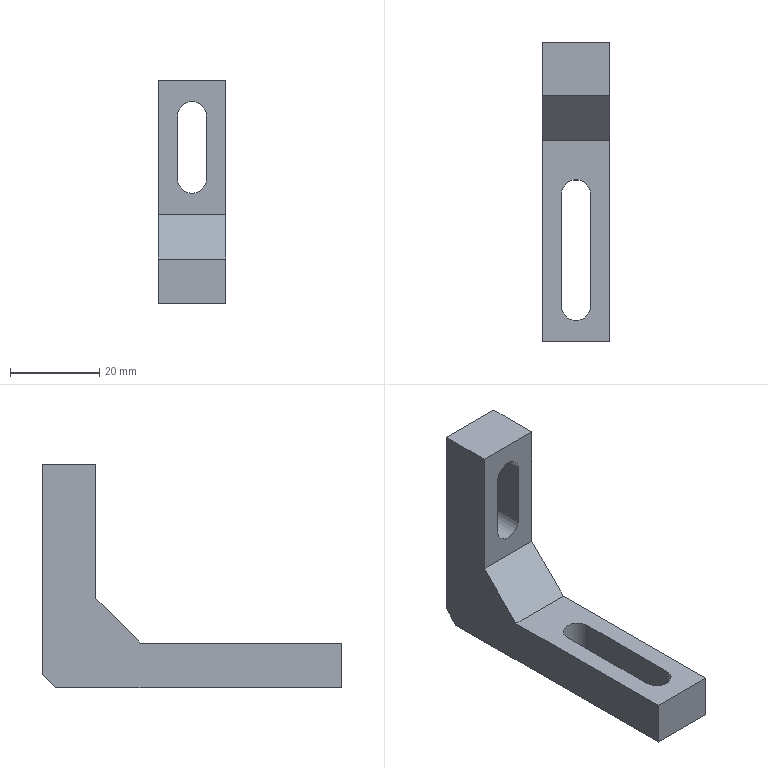Part | STEP file | 1-S938U-100524-006 | 1 solid | 18 faces | box 15 x 67 x 50 mm | volume 14485 mm3 | plane 14 | cylinder 4 | commonest cylinder face diameters 6.5 x4
STEP:
#1=CARTESIAN_POINT('',(3.25,-25.5,0.));
#2=VERTEX_POINT('',#1);
#3=CARTESIAN_POINT('',(3.25,-0.5,0.));
#4=VERTEX_POINT('',#3);
#5=CARTESIAN_POINT('',(3.25,-0.25,0.));
#6=DIRECTION('',(0.,1.,0.));
#7=VECTOR('',#6,10.);
#8=LINE('',#5,#7);
#9=EDGE_CURVE('',#2,#4,#8,.T.);
#10=ORIENTED_EDGE('',*,*,#9,.F.);
#11=CARTESIAN_POINT('',(3.25,-25.5,10.));
#12=VERTEX_POINT('',#11);
#13=CARTESIAN_POINT('',(3.25,-25.5,10.));
#14=DIRECTION('',(0.,0.,-1.));
#15=VECTOR('',#14,10.);
#16=LINE('',#13,#15);
#17=EDGE_CURVE('',#12,#2,#16,.T.);
#18=ORIENTED_EDGE('',*,*,#17,.F.);
#19=CARTESIAN_POINT('',(3.25,-0.5,10.));
#20=VERTEX_POINT('',#19);
#21=CARTESIAN_POINT('',(3.25,-0.25,10.));
#22=DIRECTION('',(0.,-1.,0.));
#23=VECTOR('',#22,10.);
#24=LINE('',#21,#23);
#25=EDGE_CURVE('',#20,#12,#24,.T.);
#26=ORIENTED_EDGE('',*,*,#25,.F.);
#27=CARTESIAN_POINT('',(3.25,-0.5,10.));
#28=DIRECTION('',(0.,0.,-1.));
#29=VECTOR('',#28,10.);
#30=LINE('',#27,#29);
#31=EDGE_CURVE('',#20,#4,#30,.T.);
#32=ORIENTED_EDGE('',*,*,#31,.T.);
#33=EDGE_LOOP('',(#10,#18,#26,#32));
#34=FACE_OUTER_BOUND('',#33,.T.);
#35=CARTESIAN_POINT('',(3.25,-0.5,10.));
#36=DIRECTION('',(1.,0.,0.));
#37=DIRECTION('',(0.,-1.,0.));
#38=AXIS2_PLACEMENT_3D('',#35,#36,#37);
#39=PLANE('',#38);
#40=ADVANCED_FACE('',(#34),#39,.F.);
#41=CARTESIAN_POINT('',(-3.25,-0.5,0.));
#42=VERTEX_POINT('',#41);
#43=CARTESIAN_POINT('',(0.,-0.5,0.));
#44=DIRECTION('',(0.,0.,1.));
#45=DIRECTION('',(1.,0.,0.));
#46=AXIS2_PLACEMENT_3D('',#43,#44,#45);
#47=CIRCLE('',#46,3.25);
#48=EDGE_CURVE('',#4,#42,#47,.T.);
#49=ORIENTED_EDGE('',*,*,#48,.F.);
#50=ORIENTED_EDGE('',*,*,#31,.F.);
#51=CARTESIAN_POINT('',(-3.25,-0.5,10.));
#52=VERTEX_POINT('',#51);
#53=CARTESIAN_POINT('',(0.,-0.5,10.));
#54=DIRECTION('',(0.,0.,-1.));
#55=DIRECTION('',(1.,0.,0.));
#56=AXIS2_PLACEMENT_3D('',#53,#54,#55);
#57=CIRCLE('',#56,3.25);
#58=EDGE_CURVE('',#52,#20,#57,.T.);
#59=ORIENTED_EDGE('',*,*,#58,.F.);
#60=CARTESIAN_POINT('',(-3.25,-0.5,10.));
#61=DIRECTION('',(0.,0.,-1.));
#62=VECTOR('',#61,10.);
#63=LINE('',#60,#62);
#64=EDGE_CURVE('',#52,#42,#63,.T.);
#65=ORIENTED_EDGE('',*,*,#64,.T.);
#66=EDGE_LOOP('',(#49,#50,#59,#65));
#67=FACE_OUTER_BOUND('',#66,.T.);
#68=CARTESIAN_POINT('',(0.,-0.5,10.));
#69=DIRECTION('',(0.,0.,-1.));
#70=DIRECTION('',(1.,0.,0.));
#71=AXIS2_PLACEMENT_3D('',#68,#69,#70);
#72=CYLINDRICAL_SURFACE('',#71,3.25);
#73=ADVANCED_FACE('',(#67),#72,.F.);
#74=CARTESIAN_POINT('',(-3.25,-25.5,0.));
#75=VERTEX_POINT('',#74);
#76=CARTESIAN_POINT('',(-3.25,-12.75,0.));
#77=DIRECTION('',(0.,-1.,0.));
#78=VECTOR('',#77,10.);
#79=LINE('',#76,#78);
#80=EDGE_CURVE('',#42,#75,#79,.T.);
#81=ORIENTED_EDGE('',*,*,#80,.F.);
#82=ORIENTED_EDGE('',*,*,#64,.F.);
#83=CARTESIAN_POINT('',(-3.25,-25.5,10.));
#84=VERTEX_POINT('',#83);
#85=CARTESIAN_POINT('',(-3.25,-12.75,10.));
#86=DIRECTION('',(0.,1.,0.));
#87=VECTOR('',#86,10.);
#88=LINE('',#85,#87);
#89=EDGE_CURVE('',#84,#52,#88,.T.);
#90=ORIENTED_EDGE('',*,*,#89,.F.);
#91=CARTESIAN_POINT('',(-3.25,-25.5,10.));
#92=DIRECTION('',(0.,0.,-1.));
#93=VECTOR('',#92,10.);
#94=LINE('',#91,#93);
#95=EDGE_CURVE('',#84,#75,#94,.T.);
#96=ORIENTED_EDGE('',*,*,#95,.T.);
#97=EDGE_LOOP('',(#81,#82,#90,#96));
#98=FACE_OUTER_BOUND('',#97,.T.);
#99=CARTESIAN_POINT('',(-3.25,-25.5,10.));
#100=DIRECTION('',(-1.,0.,0.));
#101=DIRECTION('',(0.,1.,0.));
#102=AXIS2_PLACEMENT_3D('',#99,#100,#101);
#103=PLANE('',#102);
#104=ADVANCED_FACE('',(#98),#103,.F.);
#105=CARTESIAN_POINT('',(0.,-25.5,0.));
#106=DIRECTION('',(0.,0.,1.));
#107=DIRECTION('',(-1.,0.,0.));
#108=AXIS2_PLACEMENT_3D('',#105,#106,#107);
#109=CIRCLE('',#108,3.25);
#110=EDGE_CURVE('',#75,#2,#109,.T.);
#111=ORIENTED_EDGE('',*,*,#110,.F.);
#112=ORIENTED_EDGE('',*,*,#95,.F.);
#113=CARTESIAN_POINT('',(0.,-25.5,10.));
#114=DIRECTION('',(0.,0.,-1.));
#115=DIRECTION('',(-1.,0.,0.));
#116=AXIS2_PLACEMENT_3D('',#113,#114,#115);
#117=CIRCLE('',#116,3.25);
#118=EDGE_CURVE('',#12,#84,#117,.T.);
#119=ORIENTED_EDGE('',*,*,#118,.F.);
#120=ORIENTED_EDGE('',*,*,#17,.T.);
#121=EDGE_LOOP('',(#111,#112,#119,#120));
#122=FACE_OUTER_BOUND('',#121,.T.);
#123=CARTESIAN_POINT('',(0.,-25.5,10.));
#124=DIRECTION('',(0.,0.,-1.));
#125=DIRECTION('',(-1.,0.,0.));
#126=AXIS2_PLACEMENT_3D('',#123,#124,#125);
#127=CYLINDRICAL_SURFACE('',#126,3.25);
#128=ADVANCED_FACE('',(#122),#127,.F.);
#129=CARTESIAN_POINT('',(-3.25,33.5,42.));
#130=VERTEX_POINT('',#129);
#131=CARTESIAN_POINT('',(-3.25,33.5,28.));
#132=VERTEX_POINT('',#131);
#133=CARTESIAN_POINT('',(-3.25,33.5,14.));
#134=DIRECTION('',(0.,0.,-1.));
#135=VECTOR('',#134,10.);
#136=LINE('',#133,#135);
#137=EDGE_CURVE('',#130,#132,#136,.T.);
#138=ORIENTED_EDGE('',*,*,#137,.F.);
#139=CARTESIAN_POINT('',(-3.25,21.5,42.));
#140=VERTEX_POINT('',#139);
#141=CARTESIAN_POINT('',(-3.25,21.5,42.));
#142=DIRECTION('',(0.,1.,0.));
#143=VECTOR('',#142,10.);
#144=LINE('',#141,#143);
#145=EDGE_CURVE('',#140,#130,#144,.T.);
#146=ORIENTED_EDGE('',*,*,#145,.F.);
#147=CARTESIAN_POINT('',(-3.25,21.5,28.));
#148=VERTEX_POINT('',#147);
#149=CARTESIAN_POINT('',(-3.25,21.5,19.));
#150=DIRECTION('',(0.,0.,1.));
#151=VECTOR('',#150,10.);
#152=LINE('',#149,#151);
#153=EDGE_CURVE('',#148,#140,#152,.T.);
#154=ORIENTED_EDGE('',*,*,#153,.F.);
#155=CARTESIAN_POINT('',(-3.25,21.5,28.));
#156=DIRECTION('',(0.,1.,0.));
#157=VECTOR('',#156,10.);
#158=LINE('',#155,#157);
#159=EDGE_CURVE('',#148,#132,#158,.T.);
#160=ORIENTED_EDGE('',*,*,#159,.T.);
#161=EDGE_LOOP('',(#138,#146,#154,#160));
#162=FACE_OUTER_BOUND('',#161,.T.);
#163=CARTESIAN_POINT('',(-3.25,21.5,28.));
#164=DIRECTION('',(-1.,0.,0.));
#165=DIRECTION('',(0.,0.,1.));
#166=AXIS2_PLACEMENT_3D('',#163,#164,#165);
#167=PLANE('',#166);
#168=ADVANCED_FACE('',(#162),#167,.F.);
#169=CARTESIAN_POINT('',(3.25,33.5,28.));
#170=VERTEX_POINT('',#169);
#171=CARTESIAN_POINT('',(0.,33.5,28.));
#172=DIRECTION('',(0.,-1.,0.));
#173=DIRECTION('',(-1.,0.,0.));
#174=AXIS2_PLACEMENT_3D('',#171,#172,#173);
#175=CIRCLE('',#174,3.25);
#176=EDGE_CURVE('',#132,#170,#175,.T.);
#177=ORIENTED_EDGE('',*,*,#176,.F.);
#178=ORIENTED_EDGE('',*,*,#159,.F.);
#179=CARTESIAN_POINT('',(3.25,21.5,28.));
#180=VERTEX_POINT('',#179);
#181=CARTESIAN_POINT('',(0.,21.5,28.));
#182=DIRECTION('',(0.,1.,0.));
#183=DIRECTION('',(-1.,0.,0.));
#184=AXIS2_PLACEMENT_3D('',#181,#182,#183);
#185=CIRCLE('',#184,3.25);
#186=EDGE_CURVE('',#180,#148,#185,.T.);
#187=ORIENTED_EDGE('',*,*,#186,.F.);
#188=CARTESIAN_POINT('',(3.25,21.5,28.));
#189=DIRECTION('',(0.,1.,0.));
#190=VECTOR('',#189,10.);
#191=LINE('',#188,#190);
#192=EDGE_CURVE('',#180,#170,#191,.T.);
#193=ORIENTED_EDGE('',*,*,#192,.T.);
#194=EDGE_LOOP('',(#177,#178,#187,#193));
#195=FACE_OUTER_BOUND('',#194,.T.);
#196=CARTESIAN_POINT('',(0.,21.5,28.));
#197=DIRECTION('',(0.,1.,0.));
#198=DIRECTION('',(-1.,0.,0.));
#199=AXIS2_PLACEMENT_3D('',#196,#197,#198);
#200=CYLINDRICAL_SURFACE('',#199,3.25);
#201=ADVANCED_FACE('',(#195),#200,.F.);
#202=CARTESIAN_POINT('',(3.25,33.5,42.));
#203=VERTEX_POINT('',#202);
#204=CARTESIAN_POINT('',(3.25,33.5,21.));
#205=DIRECTION('',(0.,0.,1.));
#206=VECTOR('',#205,10.);
#207=LINE('',#204,#206);
#208=EDGE_CURVE('',#170,#203,#207,.T.);
#209=ORIENTED_EDGE('',*,*,#208,.F.);
#210=ORIENTED_EDGE('',*,*,#192,.F.);
#211=CARTESIAN_POINT('',(3.25,21.5,42.));
#212=VERTEX_POINT('',#211);
#213=CARTESIAN_POINT('',(3.25,21.5,26.));
#214=DIRECTION('',(0.,0.,-1.));
#215=VECTOR('',#214,10.);
#216=LINE('',#213,#215);
#217=EDGE_CURVE('',#212,#180,#216,.T.);
#218=ORIENTED_EDGE('',*,*,#217,.F.);
#219=CARTESIAN_POINT('',(3.25,21.5,42.));
#220=DIRECTION('',(0.,1.,0.));
#221=VECTOR('',#220,10.);
#222=LINE('',#219,#221);
#223=EDGE_CURVE('',#212,#203,#222,.T.);
#224=ORIENTED_EDGE('',*,*,#223,.T.);
#225=EDGE_LOOP('',(#209,#210,#218,#224));
#226=FACE_OUTER_BOUND('',#225,.T.);
#227=CARTESIAN_POINT('',(3.25,21.5,42.));
#228=DIRECTION('',(1.,0.,0.));
#229=DIRECTION('',(0.,0.,-1.));
#230=AXIS2_PLACEMENT_3D('',#227,#228,#229);
#231=PLANE('',#230);
#232=ADVANCED_FACE('',(#226),#231,.F.);
#233=CARTESIAN_POINT('',(0.,33.5,42.));
#234=DIRECTION('',(0.,-1.,0.));
#235=DIRECTION('',(1.,0.,0.));
#236=AXIS2_PLACEMENT_3D('',#233,#234,#235);
#237=CIRCLE('',#236,3.25);
#238=EDGE_CURVE('',#203,#130,#237,.T.);
#239=ORIENTED_EDGE('',*,*,#238,.F.);
#240=ORIENTED_EDGE('',*,*,#223,.F.);
#241=CARTESIAN_POINT('',(0.,21.5,42.));
#242=DIRECTION('',(0.,1.,0.));
#243=DIRECTION('',(1.,0.,0.));
#244=AXIS2_PLACEMENT_3D('',#241,#242,#243);
#245=CIRCLE('',#244,3.25);
#246=EDGE_CURVE('',#140,#212,#245,.T.);
#247=ORIENTED_EDGE('',*,*,#246,.F.);
#248=ORIENTED_EDGE('',*,*,#145,.T.);
#249=EDGE_LOOP('',(#239,#240,#247,#248));
#250=FACE_OUTER_BOUND('',#249,.T.);
#251=CARTESIAN_POINT('',(0.,21.5,42.));
#252=DIRECTION('',(0.,1.,0.));
#253=DIRECTION('',(1.,0.,0.));
#254=AXIS2_PLACEMENT_3D('',#251,#252,#253);
#255=CYLINDRICAL_SURFACE('',#254,3.25);
#256=ADVANCED_FACE('',(#250),#255,.F.);
#257=CARTESIAN_POINT('',(-7.5,30.5,0.));
#258=VERTEX_POINT('',#257);
#259=CARTESIAN_POINT('',(-7.5,33.5,3.));
#260=VERTEX_POINT('',#259);
#261=CARTESIAN_POINT('',(-7.5,32.,1.5));
#262=DIRECTION('',(0.,0.7071,0.7071));
#263=VECTOR('',#262,10.);
#264=LINE('',#261,#263);
#265=EDGE_CURVE('',#258,#260,#264,.T.);
#266=ORIENTED_EDGE('',*,*,#265,.T.);
#267=CARTESIAN_POINT('',(7.5,33.5,3.));
#268=VERTEX_POINT('',#267);
#269=CARTESIAN_POINT('',(3.75,33.5,3.));
#270=DIRECTION('',(1.,0.,0.));
#271=VECTOR('',#270,10.);
#272=LINE('',#269,#271);
#273=EDGE_CURVE('',#260,#268,#272,.T.);
#274=ORIENTED_EDGE('',*,*,#273,.T.);
#275=CARTESIAN_POINT('',(7.5,30.5,0.));
#276=VERTEX_POINT('',#275);
#277=CARTESIAN_POINT('',(7.5,15.25,-15.25));
#278=DIRECTION('',(0.,-0.7071,-0.7071));
#279=VECTOR('',#278,10.);
#280=LINE('',#277,#279);
#281=EDGE_CURVE('',#268,#276,#280,.T.);
#282=ORIENTED_EDGE('',*,*,#281,.T.);
#283=CARTESIAN_POINT('',(3.75,30.5,0.));
#284=DIRECTION('',(-1.,0.,0.));
#285=VECTOR('',#284,10.);
#286=LINE('',#283,#285);
#287=EDGE_CURVE('',#276,#258,#286,.T.);
#288=ORIENTED_EDGE('',*,*,#287,.T.);
#289=EDGE_LOOP('',(#266,#274,#282,#288));
#290=FACE_OUTER_BOUND('',#289,.T.);
#291=CARTESIAN_POINT('',(3.75,32.,1.5));
#292=DIRECTION('',(0.,0.7071,-0.7071));
#293=DIRECTION('',(-1.,0.,0.));
#294=AXIS2_PLACEMENT_3D('',#291,#292,#293);
#295=PLANE('',#294);
#296=ADVANCED_FACE('',(#290),#295,.T.);
#297=ORIENTED_EDGE('',*,*,#273,.F.);
#298=CARTESIAN_POINT('',(-7.5,33.5,50.));
#299=VERTEX_POINT('',#298);
#300=CARTESIAN_POINT('',(-7.5,33.5,0.));
#301=DIRECTION('',(0.,0.,1.));
#302=VECTOR('',#301,10.);
#303=LINE('',#300,#302);
#304=EDGE_CURVE('',#260,#299,#303,.T.);
#305=ORIENTED_EDGE('',*,*,#304,.T.);
#306=CARTESIAN_POINT('',(7.5,33.5,50.));
#307=VERTEX_POINT('',#306);
#308=CARTESIAN_POINT('',(7.5,33.5,50.));
#309=DIRECTION('',(-1.,0.,0.));
#310=VECTOR('',#309,10.);
#311=LINE('',#308,#310);
#312=EDGE_CURVE('',#307,#299,#311,.T.);
#313=ORIENTED_EDGE('',*,*,#312,.F.);
#314=CARTESIAN_POINT('',(7.5,33.5,0.));
#315=DIRECTION('',(0.,0.,1.));
#316=VECTOR('',#315,10.);
#317=LINE('',#314,#316);
#318=EDGE_CURVE('',#268,#307,#317,.T.);
#319=ORIENTED_EDGE('',*,*,#318,.F.);
#320=EDGE_LOOP('',(#297,#305,#313,#319));
#321=FACE_OUTER_BOUND('',#320,.T.);
#322=ORIENTED_EDGE('',*,*,#208,.T.);
#323=ORIENTED_EDGE('',*,*,#238,.T.);
#324=ORIENTED_EDGE('',*,*,#137,.T.);
#325=ORIENTED_EDGE('',*,*,#176,.T.);
#326=EDGE_LOOP('',(#322,#323,#324,#325));
#327=FACE_BOUND('',#326,.T.);
#328=CARTESIAN_POINT('',(7.5,33.5,0.));
#329=DIRECTION('',(0.,1.,0.));
#330=DIRECTION('',(-1.,0.,0.));
#331=AXIS2_PLACEMENT_3D('',#328,#329,#330);
#332=PLANE('',#331);
#333=ADVANCED_FACE('',(#321,#327),#332,.T.);
#334=ORIENTED_EDGE('',*,*,#265,.F.);
#335=CARTESIAN_POINT('',(-7.5,-33.5,0.));
#336=VERTEX_POINT('',#335);
#337=CARTESIAN_POINT('',(-7.5,33.5,0.));
#338=DIRECTION('',(0.,-1.,0.));
#339=VECTOR('',#338,10.);
#340=LINE('',#337,#339);
#341=EDGE_CURVE('',#258,#336,#340,.T.);
#342=ORIENTED_EDGE('',*,*,#341,.T.);
#343=CARTESIAN_POINT('',(-7.5,-33.5,10.));
#344=VERTEX_POINT('',#343);
#345=CARTESIAN_POINT('',(-7.5,-33.5,0.));
#346=DIRECTION('',(0.,0.,1.));
#347=VECTOR('',#346,10.);
#348=LINE('',#345,#347);
#349=EDGE_CURVE('',#336,#344,#348,.T.);
#350=ORIENTED_EDGE('',*,*,#349,.T.);
#351=CARTESIAN_POINT('',(-7.5,11.5,10.));
#352=VERTEX_POINT('',#351);
#353=CARTESIAN_POINT('',(-7.5,33.5,10.));
#354=DIRECTION('',(0.,-1.,0.));
#355=VECTOR('',#354,10.);
#356=LINE('',#353,#355);
#357=EDGE_CURVE('',#352,#344,#356,.T.);
#358=ORIENTED_EDGE('',*,*,#357,.F.);
#359=CARTESIAN_POINT('',(-7.5,21.5,20.));
#360=VERTEX_POINT('',#359);
#361=CARTESIAN_POINT('',(-7.5,17.,15.5));
#362=DIRECTION('',(0.,-0.7071,-0.7071));
#363=VECTOR('',#362,10.);
#364=LINE('',#361,#363);
#365=EDGE_CURVE('',#360,#352,#364,.T.);
#366=ORIENTED_EDGE('',*,*,#365,.F.);
#367=CARTESIAN_POINT('',(-7.5,21.5,50.));
#368=VERTEX_POINT('',#367);
#369=CARTESIAN_POINT('',(-7.5,21.5,10.));
#370=DIRECTION('',(0.,0.,1.));
#371=VECTOR('',#370,10.);
#372=LINE('',#369,#371);
#373=EDGE_CURVE('',#360,#368,#372,.T.);
#374=ORIENTED_EDGE('',*,*,#373,.T.);
#375=CARTESIAN_POINT('',(-7.5,33.5,50.));
#376=DIRECTION('',(0.,-1.,0.));
#377=VECTOR('',#376,10.);
#378=LINE('',#375,#377);
#379=EDGE_CURVE('',#299,#368,#378,.T.);
#380=ORIENTED_EDGE('',*,*,#379,.F.);
#381=ORIENTED_EDGE('',*,*,#304,.F.);
#382=EDGE_LOOP('',(#334,#342,#350,#358,#366,#374,#380,#381));
#383=FACE_OUTER_BOUND('',#382,.T.);
#384=CARTESIAN_POINT('',(-7.5,33.5,0.));
#385=DIRECTION('',(-1.,0.,0.));
#386=DIRECTION('',(0.,-1.,0.));
#387=AXIS2_PLACEMENT_3D('',#384,#385,#386);
#388=PLANE('',#387);
#389=ADVANCED_FACE('',(#383),#388,.T.);
#390=CARTESIAN_POINT('',(7.5,11.5,10.));
#391=VERTEX_POINT('',#390);
#392=CARTESIAN_POINT('',(7.5,21.5,20.));
#393=VERTEX_POINT('',#392);
#394=CARTESIAN_POINT('',(7.5,0.25,-1.25));
#395=DIRECTION('',(0.,0.7071,0.7071));
#396=VECTOR('',#395,10.);
#397=LINE('',#394,#396);
#398=EDGE_CURVE('',#391,#393,#397,.T.);
#399=ORIENTED_EDGE('',*,*,#398,.T.);
#400=CARTESIAN_POINT('',(-3.75,21.5,20.));
#401=DIRECTION('',(-1.,0.,0.));
#402=VECTOR('',#401,10.);
#403=LINE('',#400,#402);
#404=EDGE_CURVE('',#393,#360,#403,.T.);
#405=ORIENTED_EDGE('',*,*,#404,.T.);
#406=ORIENTED_EDGE('',*,*,#365,.T.);
#407=CARTESIAN_POINT('',(-3.75,11.5,10.));
#408=DIRECTION('',(1.,0.,0.));
#409=VECTOR('',#408,10.);
#410=LINE('',#407,#409);
#411=EDGE_CURVE('',#352,#391,#410,.T.);
#412=ORIENTED_EDGE('',*,*,#411,.T.);
#413=EDGE_LOOP('',(#399,#405,#406,#412));
#414=FACE_OUTER_BOUND('',#413,.T.);
#415=CARTESIAN_POINT('',(-3.75,16.5,15.));
#416=DIRECTION('',(0.,-0.7071,0.7071));
#417=DIRECTION('',(1.,0.,0.));
#418=AXIS2_PLACEMENT_3D('',#415,#416,#417);
#419=PLANE('',#418);
#420=ADVANCED_FACE('',(#414),#419,.T.);
#421=ORIENTED_EDGE('',*,*,#404,.F.);
#422=CARTESIAN_POINT('',(7.5,21.5,50.));
#423=VERTEX_POINT('',#422);
#424=CARTESIAN_POINT('',(7.5,21.5,10.));
#425=DIRECTION('',(0.,0.,1.));
#426=VECTOR('',#425,10.);
#427=LINE('',#424,#426);
#428=EDGE_CURVE('',#393,#423,#427,.T.);
#429=ORIENTED_EDGE('',*,*,#428,.T.);
#430=CARTESIAN_POINT('',(-7.5,21.5,50.));
#431=DIRECTION('',(1.,0.,0.));
#432=VECTOR('',#431,10.);
#433=LINE('',#430,#432);
#434=EDGE_CURVE('',#368,#423,#433,.T.);
#435=ORIENTED_EDGE('',*,*,#434,.F.);
#436=ORIENTED_EDGE('',*,*,#373,.F.);
#437=EDGE_LOOP('',(#421,#429,#435,#436));
#438=FACE_OUTER_BOUND('',#437,.T.);
#439=ORIENTED_EDGE('',*,*,#217,.T.);
#440=ORIENTED_EDGE('',*,*,#186,.T.);
#441=ORIENTED_EDGE('',*,*,#153,.T.);
#442=ORIENTED_EDGE('',*,*,#246,.T.);
#443=EDGE_LOOP('',(#439,#440,#441,#442));
#444=FACE_BOUND('',#443,.T.);
#445=CARTESIAN_POINT('',(-7.5,21.5,10.));
#446=DIRECTION('',(0.,-1.,0.));
#447=DIRECTION('',(1.,0.,0.));
#448=AXIS2_PLACEMENT_3D('',#445,#446,#447);
#449=PLANE('',#448);
#450=ADVANCED_FACE('',(#438,#444),#449,.T.);
#451=ORIENTED_EDGE('',*,*,#434,.T.);
#452=CARTESIAN_POINT('',(7.5,-33.5,50.));
#453=DIRECTION('',(0.,1.,0.));
#454=VECTOR('',#453,10.);
#455=LINE('',#452,#454);
#456=EDGE_CURVE('',#423,#307,#455,.T.);
#457=ORIENTED_EDGE('',*,*,#456,.T.);
#458=ORIENTED_EDGE('',*,*,#312,.T.);
#459=ORIENTED_EDGE('',*,*,#379,.T.);
#460=EDGE_LOOP('',(#451,#457,#458,#459));
#461=FACE_OUTER_BOUND('',#460,.T.);
#462=CARTESIAN_POINT('',(0.,27.5,50.));
#463=DIRECTION('',(0.,0.,1.));
#464=DIRECTION('',(1.,0.,0.));
#465=AXIS2_PLACEMENT_3D('',#462,#463,#464);
#466=PLANE('',#465);
#467=ADVANCED_FACE('',(#461),#466,.T.);
#468=ORIENTED_EDGE('',*,*,#411,.F.);
#469=ORIENTED_EDGE('',*,*,#357,.T.);
#470=CARTESIAN_POINT('',(7.5,-33.5,10.));
#471=VERTEX_POINT('',#470);
#472=CARTESIAN_POINT('',(-7.5,-33.5,10.));
#473=DIRECTION('',(1.,0.,0.));
#474=VECTOR('',#473,10.);
#475=LINE('',#472,#474);
#476=EDGE_CURVE('',#344,#471,#475,.T.);
#477=ORIENTED_EDGE('',*,*,#476,.T.);
#478=CARTESIAN_POINT('',(7.5,-33.5,10.));
#479=DIRECTION('',(0.,1.,0.));
#480=VECTOR('',#479,10.);
#481=LINE('',#478,#480);
#482=EDGE_CURVE('',#471,#391,#481,.T.);
#483=ORIENTED_EDGE('',*,*,#482,.T.);
#484=EDGE_LOOP('',(#468,#469,#477,#483));
#485=FACE_OUTER_BOUND('',#484,.T.);
#486=ORIENTED_EDGE('',*,*,#89,.T.);
#487=ORIENTED_EDGE('',*,*,#58,.T.);
#488=ORIENTED_EDGE('',*,*,#25,.T.);
#489=ORIENTED_EDGE('',*,*,#118,.T.);
#490=EDGE_LOOP('',(#486,#487,#488,#489));
#491=FACE_BOUND('',#490,.T.);
#492=CARTESIAN_POINT('',(0.,0.,10.));
#493=DIRECTION('',(0.,0.,1.));
#494=DIRECTION('',(1.,0.,0.));
#495=AXIS2_PLACEMENT_3D('',#492,#493,#494);
#496=PLANE('',#495);
#497=ADVANCED_FACE('',(#485,#491),#496,.T.);
#498=ORIENTED_EDGE('',*,*,#281,.F.);
#499=ORIENTED_EDGE('',*,*,#318,.T.);
#500=ORIENTED_EDGE('',*,*,#456,.F.);
#501=ORIENTED_EDGE('',*,*,#428,.F.);
#502=ORIENTED_EDGE('',*,*,#398,.F.);
#503=ORIENTED_EDGE('',*,*,#482,.F.);
#504=CARTESIAN_POINT('',(7.5,-33.5,0.));
#505=VERTEX_POINT('',#504);
#506=CARTESIAN_POINT('',(7.5,-33.5,0.));
#507=DIRECTION('',(0.,0.,1.));
#508=VECTOR('',#507,10.);
#509=LINE('',#506,#508);
#510=EDGE_CURVE('',#505,#471,#509,.T.);
#511=ORIENTED_EDGE('',*,*,#510,.F.);
#512=CARTESIAN_POINT('',(7.5,-33.5,0.));
#513=DIRECTION('',(0.,1.,0.));
#514=VECTOR('',#513,10.);
#515=LINE('',#512,#514);
#516=EDGE_CURVE('',#505,#276,#515,.T.);
#517=ORIENTED_EDGE('',*,*,#516,.T.);
#518=EDGE_LOOP('',(#498,#499,#500,#501,#502,#503,#511,#517));
#519=FACE_OUTER_BOUND('',#518,.T.);
#520=CARTESIAN_POINT('',(7.5,-33.5,0.));
#521=DIRECTION('',(1.,0.,0.));
#522=DIRECTION('',(0.,1.,0.));
#523=AXIS2_PLACEMENT_3D('',#520,#521,#522);
#524=PLANE('',#523);
#525=ADVANCED_FACE('',(#519),#524,.T.);
#526=CARTESIAN_POINT('',(-7.5,-33.5,0.));
#527=DIRECTION('',(1.,0.,0.));
#528=VECTOR('',#527,10.);
#529=LINE('',#526,#528);
#530=EDGE_CURVE('',#336,#505,#529,.T.);
#531=ORIENTED_EDGE('',*,*,#530,.T.);
#532=ORIENTED_EDGE('',*,*,#510,.T.);
#533=ORIENTED_EDGE('',*,*,#476,.F.);
#534=ORIENTED_EDGE('',*,*,#349,.F.);
#535=EDGE_LOOP('',(#531,#532,#533,#534));
#536=FACE_OUTER_BOUND('',#535,.T.);
#537=CARTESIAN_POINT('',(-7.5,-33.5,0.));
#538=DIRECTION('',(0.,-1.,0.));
#539=DIRECTION('',(1.,0.,0.));
#540=AXIS2_PLACEMENT_3D('',#537,#538,#539);
#541=PLANE('',#540);
#542=ADVANCED_FACE('',(#536),#541,.T.);
#543=ORIENTED_EDGE('',*,*,#287,.F.);
#544=ORIENTED_EDGE('',*,*,#516,.F.);
#545=ORIENTED_EDGE('',*,*,#530,.F.);
#546=ORIENTED_EDGE('',*,*,#341,.F.);
#547=EDGE_LOOP('',(#543,#544,#545,#546));
#548=FACE_OUTER_BOUND('',#547,.T.);
#549=ORIENTED_EDGE('',*,*,#80,.T.);
#550=ORIENTED_EDGE('',*,*,#110,.T.);
#551=ORIENTED_EDGE('',*,*,#9,.T.);
#552=ORIENTED_EDGE('',*,*,#48,.T.);
#553=EDGE_LOOP('',(#549,#550,#551,#552));
#554=FACE_BOUND('',#553,.T.);
#555=CARTESIAN_POINT('',(0.,0.,0.));
#556=DIRECTION('',(0.,0.,1.));
#557=DIRECTION('',(1.,0.,0.));
#558=AXIS2_PLACEMENT_3D('',#555,#556,#557);
#559=PLANE('',#558);
#560=ADVANCED_FACE('',(#548,#554),#559,.F.);
#561=CLOSED_SHELL('',(#40,#73,#104,#128,#168,#201,#232,#256,#296,#333,#389,#420,#450,#467,#497,#525,#542,#560));
#562=MANIFOLD_SOLID_BREP('',#561);
#563=(LENGTH_UNIT()NAMED_UNIT(*)SI_UNIT(.MILLI.,.METRE.));
#564=UNCERTAINTY_MEASURE_WITH_UNIT(LENGTH_MEASURE(0.01),#563,'','');
#565=(NAMED_UNIT(*)PLANE_ANGLE_UNIT()SI_UNIT($,.RADIAN.));
#566=(NAMED_UNIT(*)SI_UNIT($,.STERADIAN.)SOLID_ANGLE_UNIT());
#567=(GEOMETRIC_REPRESENTATION_CONTEXT(3)GLOBAL_UNCERTAINTY_ASSIGNED_CONTEXT((#564))GLOBAL_UNIT_ASSIGNED_CONTEXT((#563,#565,#566))REPRESENTATION_CONTEXT('',''));
#568=ADVANCED_BREP_SHAPE_REPRESENTATION('',(#562),#567);